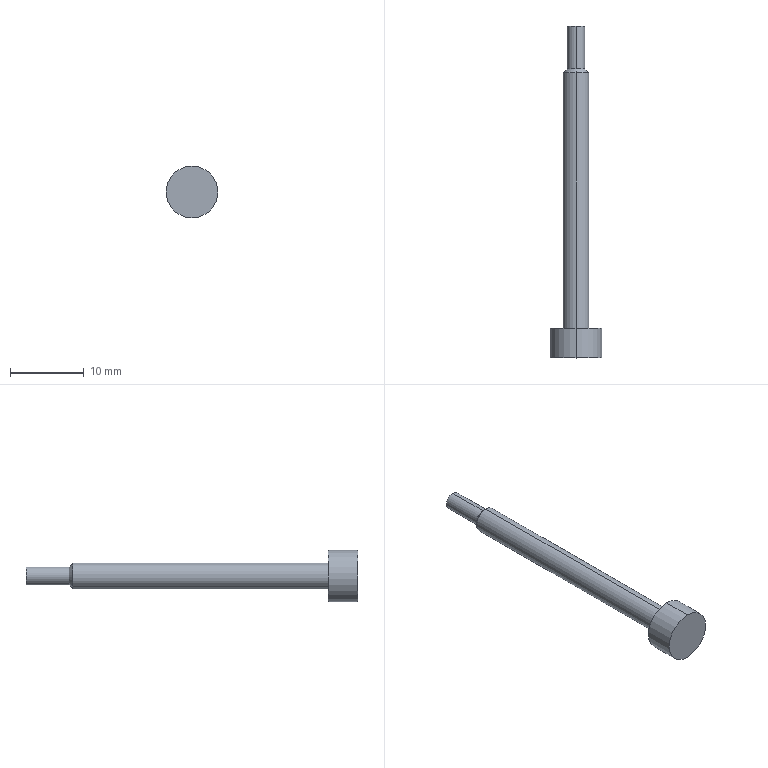Part | STEP file | 1 solid | 12 faces | box 7 x 45.025 x 7 mm | volume 517.748 mm3 | cylinder 6 | plane 4 | cone 2 | commonest cylinder face diameters 2.412 x2 3.5 x2 7 x2
STEP:
#1=CARTESIAN_POINT('',(0.,0.,0.));
#2=DIRECTION('',(0.,0.,1.));
#3=DIRECTION('',(1.,0.,0.));
#4=AXIS2_PLACEMENT_3D('',#1,#2,#3);
#5=CARTESIAN_POINT('',(-135.173,-40.,196.963));
#6=VERTEX_POINT('',#5);
#7=CARTESIAN_POINT('',(-135.173,-40.,189.963));
#8=VERTEX_POINT('',#7);
#9=CARTESIAN_POINT('',(-135.173,-40.,193.463));
#10=DIRECTION('',(0.,1.,0.));
#11=DIRECTION('',(0.,0.,-1.));
#12=AXIS2_PLACEMENT_3D('',#9,#10,#11);
#13=CIRCLE('',#12,3.5);
#14=CARTESIAN_POINT('',(-135.173,-50.,193.463));
#15=DIRECTION('',(0.,1.,0.));
#16=DIRECTION('',(0.,0.,1.));
#17=AXIS2_PLACEMENT_3D('',#14,#15,#16);
#18=CYLINDRICAL_SURFACE('',#17,3.5);
#19=CARTESIAN_POINT('',(-3.142,10.));
#20=DIRECTION('',(1.,0.));
#21=VECTOR('',#20,1.);
#22=LINE('',#19,#21);
#23=(GEOMETRIC_REPRESENTATION_CONTEXT(2)PARAMETRIC_REPRESENTATION_CONTEXT()REPRESENTATION_CONTEXT('',''));
#24=DEFINITIONAL_REPRESENTATION('',(#22),#23);
#25=PCURVE('',#18,#24);
#26=CARTESIAN_POINT('',(-72.862,-40.,23.556));
#27=DIRECTION('',(0.,-1.,0.));
#28=DIRECTION('',(0.,0.,-1.));
#29=AXIS2_PLACEMENT_3D('',#26,#27,#28);
#30=PLANE('',#29);
#31=CARTESIAN_POINT('',(-166.407,-62.31));
#32=CARTESIAN_POINT('',(-166.407,-68.372));
#33=CARTESIAN_POINT('',(-171.657,-65.341));
#34=CARTESIAN_POINT('',(-176.907,-62.31));
#35=CARTESIAN_POINT('',(-171.657,-59.279));
#36=CARTESIAN_POINT('',(-166.407,-56.248));
#37=CARTESIAN_POINT('',(-166.407,-62.31));
#38=(BOUNDED_CURVE()B_SPLINE_CURVE(2,(#31,#32,#33,#34,#35,#36,#37),.UNSPECIFIED.,.T.,.F.)B_SPLINE_CURVE_WITH_KNOTS((1,2,2,2,2,1),(-2.094,0.,2.094,4.189,6.283,8.378),.UNSPECIFIED.)CURVE()GEOMETRIC_REPRESENTATION_ITEM()RATIONAL_B_SPLINE_CURVE((1.,0.5,1.,0.5,1.,0.5,1.))REPRESENTATION_ITEM(''));
#39=(GEOMETRIC_REPRESENTATION_CONTEXT(2)PARAMETRIC_REPRESENTATION_CONTEXT()REPRESENTATION_CONTEXT('',''));
#40=DEFINITIONAL_REPRESENTATION('',(#38),#39);
#41=PCURVE('',#30,#40);
#42=SURFACE_CURVE('',#13,(#25,#41),.PCURVE_S1.);
#43=EDGE_CURVE('',#6,#8,#42,.T.);
#44=ORIENTED_EDGE('',*,*,#43,.T.);
#45=CARTESIAN_POINT('',(-135.173,-36.,189.963));
#46=VERTEX_POINT('',#45);
#47=CARTESIAN_POINT('',(-135.173,-50.,189.963));
#48=DIRECTION('',(0.,1.,0.));
#49=VECTOR('',#48,1.);
#50=LINE('',#47,#49);
#51=CARTESIAN_POINT('',(3.142,0.));
#52=DIRECTION('',(0.,1.));
#53=VECTOR('',#52,1.);
#54=LINE('',#51,#53);
#55=(GEOMETRIC_REPRESENTATION_CONTEXT(2)PARAMETRIC_REPRESENTATION_CONTEXT()REPRESENTATION_CONTEXT('',''));
#56=DEFINITIONAL_REPRESENTATION('',(#54),#55);
#57=PCURVE('',#18,#56);
#58=CARTESIAN_POINT('',(-135.173,-50.,193.463));
#59=DIRECTION('',(0.,1.,0.));
#60=DIRECTION('',(0.,0.,1.));
#61=AXIS2_PLACEMENT_3D('',#58,#59,#60);
#62=CYLINDRICAL_SURFACE('',#61,3.5);
#63=CARTESIAN_POINT('',(3.142,0.));
#64=DIRECTION('',(0.,1.));
#65=VECTOR('',#64,1.);
#66=LINE('',#63,#65);
#67=(GEOMETRIC_REPRESENTATION_CONTEXT(2)PARAMETRIC_REPRESENTATION_CONTEXT()REPRESENTATION_CONTEXT('',''));
#68=DEFINITIONAL_REPRESENTATION('',(#66),#67);
#69=PCURVE('',#62,#68);
#70=SURFACE_CURVE('',#50,(#57,#69),.PCURVE_S1.);
#71=EDGE_CURVE('',#8,#46,#70,.T.);
#72=ORIENTED_EDGE('',*,*,#71,.T.);
#73=CARTESIAN_POINT('',(-135.173,-36.,196.963));
#74=VERTEX_POINT('',#73);
#75=CARTESIAN_POINT('',(-135.173,-36.,193.463));
#76=DIRECTION('',(0.,-1.,0.));
#77=DIRECTION('',(0.,0.,-1.));
#78=AXIS2_PLACEMENT_3D('',#75,#76,#77);
#79=CIRCLE('',#78,3.5);
#80=CARTESIAN_POINT('',(3.142,14.));
#81=DIRECTION('',(-1.,0.));
#82=VECTOR('',#81,1.);
#83=LINE('',#80,#82);
#84=(GEOMETRIC_REPRESENTATION_CONTEXT(2)PARAMETRIC_REPRESENTATION_CONTEXT()REPRESENTATION_CONTEXT('',''));
#85=DEFINITIONAL_REPRESENTATION('',(#83),#84);
#86=PCURVE('',#18,#85);
#87=CARTESIAN_POINT('',(-135.173,-36.,193.463));
#88=DIRECTION('',(0.,1.,0.));
#89=DIRECTION('',(0.,0.,1.));
#90=AXIS2_PLACEMENT_3D('',#87,#88,#89);
#91=PLANE('',#90);
#92=CARTESIAN_POINT('',(-3.5,0.));
#93=CARTESIAN_POINT('',(-3.5,6.062));
#94=CARTESIAN_POINT('',(1.75,3.031));
#95=CARTESIAN_POINT('',(7.,0.));
#96=CARTESIAN_POINT('',(1.75,-3.031));
#97=CARTESIAN_POINT('',(-3.5,-6.062));
#98=CARTESIAN_POINT('',(-3.5,0.));
#99=(BOUNDED_CURVE()B_SPLINE_CURVE(2,(#92,#93,#94,#95,#96,#97,#98),.UNSPECIFIED.,.T.,.F.)B_SPLINE_CURVE_WITH_KNOTS((1,2,2,2,2,1),(-2.094,0.,2.094,4.189,6.283,8.378),.UNSPECIFIED.)CURVE()GEOMETRIC_REPRESENTATION_ITEM()RATIONAL_B_SPLINE_CURVE((1.,0.5,1.,0.5,1.,0.5,1.))REPRESENTATION_ITEM(''));
#100=(GEOMETRIC_REPRESENTATION_CONTEXT(2)PARAMETRIC_REPRESENTATION_CONTEXT()REPRESENTATION_CONTEXT('',''));
#101=DEFINITIONAL_REPRESENTATION('',(#99),#100);
#102=PCURVE('',#91,#101);
#103=SURFACE_CURVE('',#79,(#86,#102),.PCURVE_S1.);
#104=EDGE_CURVE('',#46,#74,#103,.T.);
#105=ORIENTED_EDGE('',*,*,#104,.T.);
#106=CARTESIAN_POINT('',(-135.173,-50.,196.963));
#107=DIRECTION('',(0.,1.,0.));
#108=VECTOR('',#107,1.);
#109=LINE('',#106,#108);
#110=CARTESIAN_POINT('',(0.,0.));
#111=DIRECTION('',(0.,1.));
#112=VECTOR('',#111,1.);
#113=LINE('',#110,#112);
#114=(GEOMETRIC_REPRESENTATION_CONTEXT(2)PARAMETRIC_REPRESENTATION_CONTEXT()REPRESENTATION_CONTEXT('',''));
#115=DEFINITIONAL_REPRESENTATION('',(#113),#114);
#116=PCURVE('',#18,#115);
#117=CARTESIAN_POINT('',(6.283,0.));
#118=DIRECTION('',(0.,1.));
#119=VECTOR('',#118,1.);
#120=LINE('',#117,#119);
#121=(GEOMETRIC_REPRESENTATION_CONTEXT(2)PARAMETRIC_REPRESENTATION_CONTEXT()REPRESENTATION_CONTEXT('',''));
#122=DEFINITIONAL_REPRESENTATION('',(#120),#121);
#123=PCURVE('',#62,#122);
#124=SURFACE_CURVE('',#109,(#116,#123),.PCURVE_S1.);
#125=EDGE_CURVE('',#6,#74,#124,.T.);
#126=ORIENTED_EDGE('',*,*,#125,.F.);
#127=EDGE_LOOP('',(#44,#72,#105,#126));
#128=FACE_BOUND('',#127,.T.);
#129=ADVANCED_FACE('',(#128),#18,.T.);
#130=CARTESIAN_POINT('',(-135.173,-1.306,195.213));
#131=VERTEX_POINT('',#130);
#132=CARTESIAN_POINT('',(-135.173,-1.306,191.713));
#133=VERTEX_POINT('',#132);
#134=CARTESIAN_POINT('',(-135.173,-1.306,193.463));
#135=DIRECTION('',(0.,1.,0.));
#136=DIRECTION('',(0.,0.,-1.));
#137=AXIS2_PLACEMENT_3D('',#134,#135,#136);
#138=CIRCLE('',#137,1.75);
#139=CARTESIAN_POINT('',(-135.173,5.025,193.463));
#140=DIRECTION('',(0.,-1.,0.));
#141=DIRECTION('',(0.,0.,-1.));
#142=AXIS2_PLACEMENT_3D('',#139,#140,#141);
#143=CYLINDRICAL_SURFACE('',#142,1.75);
#144=CARTESIAN_POINT('',(6.283,6.332));
#145=DIRECTION('',(-1.,0.));
#146=VECTOR('',#145,1.);
#147=LINE('',#144,#146);
#148=(GEOMETRIC_REPRESENTATION_CONTEXT(2)PARAMETRIC_REPRESENTATION_CONTEXT()REPRESENTATION_CONTEXT('',''));
#149=DEFINITIONAL_REPRESENTATION('',(#147),#148);
#150=PCURVE('',#143,#149);
#151=CARTESIAN_POINT('',(-134.168,-1.306,193.908));
#152=DIRECTION('',(0.,-1.,0.));
#153=DIRECTION('',(0.,0.,-1.));
#154=AXIS2_PLACEMENT_3D('',#151,#152,#153);
#155=PLANE('',#154);
#156=CARTESIAN_POINT('',(2.196,-1.005));
#157=CARTESIAN_POINT('',(2.196,-4.036));
#158=CARTESIAN_POINT('',(-0.4291,-2.52));
#159=CARTESIAN_POINT('',(-3.054,-1.005));
#160=CARTESIAN_POINT('',(-0.4291,0.5106));
#161=CARTESIAN_POINT('',(2.196,2.026));
#162=CARTESIAN_POINT('',(2.196,-1.005));
#163=(BOUNDED_CURVE()B_SPLINE_CURVE(2,(#156,#157,#158,#159,#160,#161,#162),.UNSPECIFIED.,.T.,.F.)B_SPLINE_CURVE_WITH_KNOTS((1,2,2,2,2,1),(-2.094,0.,2.094,4.189,6.283,8.378),.UNSPECIFIED.)CURVE()GEOMETRIC_REPRESENTATION_ITEM()RATIONAL_B_SPLINE_CURVE((1.,0.5,1.,0.5,1.,0.5,1.))REPRESENTATION_ITEM(''));
#164=(GEOMETRIC_REPRESENTATION_CONTEXT(2)PARAMETRIC_REPRESENTATION_CONTEXT()REPRESENTATION_CONTEXT('',''));
#165=DEFINITIONAL_REPRESENTATION('',(#163),#164);
#166=PCURVE('',#155,#165);
#167=SURFACE_CURVE('',#138,(#150,#166),.PCURVE_S1.);
#168=EDGE_CURVE('',#131,#133,#167,.T.);
#169=ORIENTED_EDGE('',*,*,#168,.F.);
#170=CARTESIAN_POINT('',(-135.173,-36.,195.213));
#171=VERTEX_POINT('',#170);
#172=CARTESIAN_POINT('',(-135.173,5.025,195.213));
#173=DIRECTION('',(0.,-1.,0.));
#174=VECTOR('',#173,1.);
#175=LINE('',#172,#174);
#176=CARTESIAN_POINT('',(3.142,0.));
#177=DIRECTION('',(0.,1.));
#178=VECTOR('',#177,1.);
#179=LINE('',#176,#178);
#180=(GEOMETRIC_REPRESENTATION_CONTEXT(2)PARAMETRIC_REPRESENTATION_CONTEXT()REPRESENTATION_CONTEXT('',''));
#181=DEFINITIONAL_REPRESENTATION('',(#179),#180);
#182=PCURVE('',#143,#181);
#183=CARTESIAN_POINT('',(-135.173,5.025,193.463));
#184=DIRECTION('',(0.,-1.,0.));
#185=DIRECTION('',(0.,0.,-1.));
#186=AXIS2_PLACEMENT_3D('',#183,#184,#185);
#187=CYLINDRICAL_SURFACE('',#186,1.75);
#188=CARTESIAN_POINT('',(3.142,0.));
#189=DIRECTION('',(0.,1.));
#190=VECTOR('',#189,1.);
#191=LINE('',#188,#190);
#192=(GEOMETRIC_REPRESENTATION_CONTEXT(2)PARAMETRIC_REPRESENTATION_CONTEXT()REPRESENTATION_CONTEXT('',''));
#193=DEFINITIONAL_REPRESENTATION('',(#191),#192);
#194=PCURVE('',#187,#193);
#195=SURFACE_CURVE('',#175,(#182,#194),.PCURVE_S1.);
#196=EDGE_CURVE('',#131,#171,#195,.T.);
#197=ORIENTED_EDGE('',*,*,#196,.T.);
#198=CARTESIAN_POINT('',(-135.173,-36.,191.713));
#199=VERTEX_POINT('',#198);
#200=CARTESIAN_POINT('',(-135.173,-36.,193.463));
#201=DIRECTION('',(0.,-1.,0.));
#202=DIRECTION('',(0.,0.,1.));
#203=AXIS2_PLACEMENT_3D('',#200,#201,#202);
#204=CIRCLE('',#203,1.75);
#205=CARTESIAN_POINT('',(-3.142,41.025));
#206=DIRECTION('',(1.,0.));
#207=VECTOR('',#206,1.);
#208=LINE('',#205,#207);
#209=(GEOMETRIC_REPRESENTATION_CONTEXT(2)PARAMETRIC_REPRESENTATION_CONTEXT()REPRESENTATION_CONTEXT('',''));
#210=DEFINITIONAL_REPRESENTATION('',(#208),#209);
#211=PCURVE('',#143,#210);
#212=CARTESIAN_POINT('',(1.75,0.));
#213=CARTESIAN_POINT('',(1.75,-3.031));
#214=CARTESIAN_POINT('',(-0.875,-1.516));
#215=CARTESIAN_POINT('',(-3.5,0.));
#216=CARTESIAN_POINT('',(-0.875,1.516));
#217=CARTESIAN_POINT('',(1.75,3.031));
#218=CARTESIAN_POINT('',(1.75,0.));
#219=(BOUNDED_CURVE()B_SPLINE_CURVE(2,(#212,#213,#214,#215,#216,#217,#218),.UNSPECIFIED.,.T.,.F.)B_SPLINE_CURVE_WITH_KNOTS((1,2,2,2,2,1),(-2.094,0.,2.094,4.189,6.283,8.378),.UNSPECIFIED.)CURVE()GEOMETRIC_REPRESENTATION_ITEM()RATIONAL_B_SPLINE_CURVE((1.,0.5,1.,0.5,1.,0.5,1.))REPRESENTATION_ITEM(''));
#220=(GEOMETRIC_REPRESENTATION_CONTEXT(2)PARAMETRIC_REPRESENTATION_CONTEXT()REPRESENTATION_CONTEXT('',''));
#221=DEFINITIONAL_REPRESENTATION('',(#219),#220);
#222=PCURVE('',#91,#221);
#223=SURFACE_CURVE('',#204,(#211,#222),.PCURVE_S1.);
#224=EDGE_CURVE('',#199,#171,#223,.T.);
#225=ORIENTED_EDGE('',*,*,#224,.F.);
#226=CARTESIAN_POINT('',(-135.173,5.025,191.713));
#227=DIRECTION('',(0.,-1.,0.));
#228=VECTOR('',#227,1.);
#229=LINE('',#226,#228);
#230=CARTESIAN_POINT('',(0.,0.));
#231=DIRECTION('',(0.,1.));
#232=VECTOR('',#231,1.);
#233=LINE('',#230,#232);
#234=(GEOMETRIC_REPRESENTATION_CONTEXT(2)PARAMETRIC_REPRESENTATION_CONTEXT()REPRESENTATION_CONTEXT('',''));
#235=DEFINITIONAL_REPRESENTATION('',(#233),#234);
#236=PCURVE('',#143,#235);
#237=CARTESIAN_POINT('',(6.283,0.));
#238=DIRECTION('',(0.,1.));
#239=VECTOR('',#238,1.);
#240=LINE('',#237,#239);
#241=(GEOMETRIC_REPRESENTATION_CONTEXT(2)PARAMETRIC_REPRESENTATION_CONTEXT()REPRESENTATION_CONTEXT('',''));
#242=DEFINITIONAL_REPRESENTATION('',(#240),#241);
#243=PCURVE('',#187,#242);
#244=SURFACE_CURVE('',#229,(#236,#243),.PCURVE_S1.);
#245=EDGE_CURVE('',#133,#199,#244,.T.);
#246=ORIENTED_EDGE('',*,*,#245,.F.);
#247=EDGE_LOOP('',(#169,#197,#225,#246));
#248=FACE_BOUND('',#247,.T.);
#249=ADVANCED_FACE('',(#248),#143,.T.);
#250=CARTESIAN_POINT('',(-135.173,-0.804,192.256));
#251=VERTEX_POINT('',#250);
#252=CARTESIAN_POINT('',(-135.173,-0.804,194.668));
#253=VERTEX_POINT('',#252);
#254=CARTESIAN_POINT('',(-135.173,-0.804,193.463));
#255=DIRECTION('',(0.,-1.,0.));
#256=DIRECTION('',(0.,0.,-1.));
#257=AXIS2_PLACEMENT_3D('',#254,#255,#256);
#258=CIRCLE('',#257,1.206);
#259=CARTESIAN_POINT('',(-135.173,-1.306,193.463));
#260=DIRECTION('',(0.,-1.,0.));
#261=DIRECTION('',(0.,0.,-1.));
#262=AXIS2_PLACEMENT_3D('',#259,#260,#261);
#263=CONICAL_SURFACE('',#262,1.708,0.7854);
#264=CARTESIAN_POINT('',(0.,-0.5025));
#265=DIRECTION('',(1.,0.));
#266=VECTOR('',#265,1.);
#267=LINE('',#264,#266);
#268=(GEOMETRIC_REPRESENTATION_CONTEXT(2)PARAMETRIC_REPRESENTATION_CONTEXT()REPRESENTATION_CONTEXT('',''));
#269=DEFINITIONAL_REPRESENTATION('',(#267),#268);
#270=PCURVE('',#263,#269);
#271=CARTESIAN_POINT('',(-135.173,90.286,193.463));
#272=DIRECTION('',(0.,-1.,0.));
#273=DIRECTION('',(0.,0.,-1.));
#274=AXIS2_PLACEMENT_3D('',#271,#272,#273);
#275=CYLINDRICAL_SURFACE('',#274,1.206);
#276=CARTESIAN_POINT('',(0.,91.09));
#277=DIRECTION('',(1.,0.));
#278=VECTOR('',#277,1.);
#279=LINE('',#276,#278);
#280=(GEOMETRIC_REPRESENTATION_CONTEXT(2)PARAMETRIC_REPRESENTATION_CONTEXT()REPRESENTATION_CONTEXT('',''));
#281=DEFINITIONAL_REPRESENTATION('',(#279),#280);
#282=PCURVE('',#275,#281);
#283=SURFACE_CURVE('',#258,(#270,#282),.PCURVE_S1.);
#284=EDGE_CURVE('',#251,#253,#283,.T.);
#285=ORIENTED_EDGE('',*,*,#284,.T.);
#286=CARTESIAN_POINT('',(-135.173,-1.306,195.171));
#287=VERTEX_POINT('',#286);
#288=CARTESIAN_POINT('',(-135.173,-1.306,195.171));
#289=DIRECTION('',(0.,-0.7071,0.7071));
#290=VECTOR('',#289,1.);
#291=LINE('',#288,#290);
#292=CARTESIAN_POINT('',(3.142,0.));
#293=DIRECTION('',(0.,1.));
#294=VECTOR('',#293,1.);
#295=LINE('',#292,#294);
#296=(GEOMETRIC_REPRESENTATION_CONTEXT(2)PARAMETRIC_REPRESENTATION_CONTEXT()REPRESENTATION_CONTEXT('',''));
#297=DEFINITIONAL_REPRESENTATION('',(#295),#296);
#298=PCURVE('',#263,#297);
#299=CARTESIAN_POINT('',(-135.173,-1.306,193.463));
#300=DIRECTION('',(0.,-1.,0.));
#301=DIRECTION('',(0.,0.,-1.));
#302=AXIS2_PLACEMENT_3D('',#299,#300,#301);
#303=CONICAL_SURFACE('',#302,1.708,0.7854);
#304=CARTESIAN_POINT('',(3.142,0.));
#305=DIRECTION('',(0.,1.));
#306=VECTOR('',#305,1.);
#307=LINE('',#304,#306);
#308=(GEOMETRIC_REPRESENTATION_CONTEXT(2)PARAMETRIC_REPRESENTATION_CONTEXT()REPRESENTATION_CONTEXT('',''));
#309=DEFINITIONAL_REPRESENTATION('',(#307),#308);
#310=PCURVE('',#303,#309);
#311=SURFACE_CURVE('',#291,(#298,#310),.PCURVE_S1.);
#312=EDGE_CURVE('',#253,#287,#311,.T.);
#313=ORIENTED_EDGE('',*,*,#312,.T.);
#314=CARTESIAN_POINT('',(-135.173,-1.306,191.754));
#315=VERTEX_POINT('',#314);
#316=CARTESIAN_POINT('',(-135.173,-1.306,193.463));
#317=DIRECTION('',(0.,1.,0.));
#318=DIRECTION('',(0.,0.,-1.));
#319=AXIS2_PLACEMENT_3D('',#316,#317,#318);
#320=CIRCLE('',#319,1.708);
#321=CARTESIAN_POINT('',(6.283,0.));
#322=DIRECTION('',(-1.,0.));
#323=VECTOR('',#322,1.);
#324=LINE('',#321,#323);
#325=(GEOMETRIC_REPRESENTATION_CONTEXT(2)PARAMETRIC_REPRESENTATION_CONTEXT()REPRESENTATION_CONTEXT('',''));
#326=DEFINITIONAL_REPRESENTATION('',(#324),#325);
#327=PCURVE('',#263,#326);
#328=CARTESIAN_POINT('',(2.154,-1.005));
#329=CARTESIAN_POINT('',(2.154,-3.964));
#330=CARTESIAN_POINT('',(-0.4083,-2.485));
#331=CARTESIAN_POINT('',(-2.971,-1.005));
#332=CARTESIAN_POINT('',(-0.4083,0.4747));
#333=CARTESIAN_POINT('',(2.154,1.954));
#334=CARTESIAN_POINT('',(2.154,-1.005));
#335=(BOUNDED_CURVE()B_SPLINE_CURVE(2,(#328,#329,#330,#331,#332,#333,#334),.UNSPECIFIED.,.T.,.F.)B_SPLINE_CURVE_WITH_KNOTS((1,2,2,2,2,1),(-2.094,0.,2.094,4.189,6.283,8.378),.UNSPECIFIED.)CURVE()GEOMETRIC_REPRESENTATION_ITEM()RATIONAL_B_SPLINE_CURVE((1.,0.5,1.,0.5,1.,0.5,1.))REPRESENTATION_ITEM(''));
#336=(GEOMETRIC_REPRESENTATION_CONTEXT(2)PARAMETRIC_REPRESENTATION_CONTEXT()REPRESENTATION_CONTEXT('',''));
#337=DEFINITIONAL_REPRESENTATION('',(#335),#336);
#338=PCURVE('',#155,#337);
#339=SURFACE_CURVE('',#320,(#327,#338),.PCURVE_S1.);
#340=EDGE_CURVE('',#287,#315,#339,.T.);
#341=ORIENTED_EDGE('',*,*,#340,.T.);
#342=CARTESIAN_POINT('',(-135.173,-1.306,191.754));
#343=DIRECTION('',(0.,-0.7071,-0.7071));
#344=VECTOR('',#343,1.);
#345=LINE('',#342,#344);
#346=CARTESIAN_POINT('',(0.,0.));
#347=DIRECTION('',(0.,1.));
#348=VECTOR('',#347,1.);
#349=LINE('',#346,#348);
#350=(GEOMETRIC_REPRESENTATION_CONTEXT(2)PARAMETRIC_REPRESENTATION_CONTEXT()REPRESENTATION_CONTEXT('',''));
#351=DEFINITIONAL_REPRESENTATION('',(#349),#350);
#352=PCURVE('',#263,#351);
#353=CARTESIAN_POINT('',(6.283,0.));
#354=DIRECTION('',(0.,1.));
#355=VECTOR('',#354,1.);
#356=LINE('',#353,#355);
#357=(GEOMETRIC_REPRESENTATION_CONTEXT(2)PARAMETRIC_REPRESENTATION_CONTEXT()REPRESENTATION_CONTEXT('',''));
#358=DEFINITIONAL_REPRESENTATION('',(#356),#357);
#359=PCURVE('',#303,#358);
#360=SURFACE_CURVE('',#345,(#352,#359),.PCURVE_S1.);
#361=EDGE_CURVE('',#251,#315,#360,.T.);
#362=ORIENTED_EDGE('',*,*,#361,.F.);
#363=EDGE_LOOP('',(#285,#313,#341,#362));
#364=FACE_BOUND('',#363,.T.);
#365=ADVANCED_FACE('',(#364),#263,.T.);
#366=CARTESIAN_POINT('',(-135.173,5.025,194.668));
#367=VERTEX_POINT('',#366);
#368=CARTESIAN_POINT('',(-135.173,5.025,192.256));
#369=VERTEX_POINT('',#368);
#370=CARTESIAN_POINT('',(-135.173,5.025,193.463));
#371=DIRECTION('',(0.,1.,0.));
#372=DIRECTION('',(0.,0.,1.));
#373=AXIS2_PLACEMENT_3D('',#370,#371,#372);
#374=CIRCLE('',#373,1.206);
#375=CARTESIAN_POINT('',(3.142,85.261));
#376=DIRECTION('',(-1.,0.));
#377=VECTOR('',#376,1.);
#378=LINE('',#375,#377);
#379=(GEOMETRIC_REPRESENTATION_CONTEXT(2)PARAMETRIC_REPRESENTATION_CONTEXT()REPRESENTATION_CONTEXT('',''));
#380=DEFINITIONAL_REPRESENTATION('',(#378),#379);
#381=PCURVE('',#275,#380);
#382=CARTESIAN_POINT('',(-135.173,5.025,193.463));
#383=DIRECTION('',(0.,1.,0.));
#384=DIRECTION('',(0.,0.,1.));
#385=AXIS2_PLACEMENT_3D('',#382,#383,#384);
#386=PLANE('',#385);
#387=CARTESIAN_POINT('',(0.,0.));
#388=DIRECTION('',(1.,0.));
#389=AXIS2_PLACEMENT_2D('',#387,#388);
#390=CIRCLE('',#389,1.206);
#391=(GEOMETRIC_REPRESENTATION_CONTEXT(2)PARAMETRIC_REPRESENTATION_CONTEXT()REPRESENTATION_CONTEXT('',''));
#392=DEFINITIONAL_REPRESENTATION('',(#390),#391);
#393=PCURVE('',#386,#392);
#394=SURFACE_CURVE('',#374,(#381,#393),.PCURVE_S1.);
#395=EDGE_CURVE('',#367,#369,#394,.T.);
#396=ORIENTED_EDGE('',*,*,#395,.F.);
#397=CARTESIAN_POINT('',(-135.173,90.286,194.668));
#398=DIRECTION('',(0.,-1.,0.));
#399=VECTOR('',#398,1.);
#400=LINE('',#397,#399);
#401=CARTESIAN_POINT('',(3.142,0.));
#402=DIRECTION('',(0.,1.));
#403=VECTOR('',#402,1.);
#404=LINE('',#401,#403);
#405=(GEOMETRIC_REPRESENTATION_CONTEXT(2)PARAMETRIC_REPRESENTATION_CONTEXT()REPRESENTATION_CONTEXT('',''));
#406=DEFINITIONAL_REPRESENTATION('',(#404),#405);
#407=PCURVE('',#275,#406);
#408=CARTESIAN_POINT('',(-135.173,90.286,193.463));
#409=DIRECTION('',(0.,-1.,0.));
#410=DIRECTION('',(0.,0.,-1.));
#411=AXIS2_PLACEMENT_3D('',#408,#409,#410);
#412=CYLINDRICAL_SURFACE('',#411,1.206);
#413=CARTESIAN_POINT('',(3.142,0.));
#414=DIRECTION('',(0.,1.));
#415=VECTOR('',#414,1.);
#416=LINE('',#413,#415);
#417=(GEOMETRIC_REPRESENTATION_CONTEXT(2)PARAMETRIC_REPRESENTATION_CONTEXT()REPRESENTATION_CONTEXT('',''));
#418=DEFINITIONAL_REPRESENTATION('',(#416),#417);
#419=PCURVE('',#412,#418);
#420=SURFACE_CURVE('',#400,(#407,#419),.PCURVE_S1.);
#421=EDGE_CURVE('',#367,#253,#420,.T.);
#422=ORIENTED_EDGE('',*,*,#421,.T.);
#423=ORIENTED_EDGE('',*,*,#284,.F.);
#424=CARTESIAN_POINT('',(-135.173,90.286,192.256));
#425=DIRECTION('',(0.,-1.,0.));
#426=VECTOR('',#425,1.);
#427=LINE('',#424,#426);
#428=CARTESIAN_POINT('',(0.,0.));
#429=DIRECTION('',(0.,1.));
#430=VECTOR('',#429,1.);
#431=LINE('',#428,#430);
#432=(GEOMETRIC_REPRESENTATION_CONTEXT(2)PARAMETRIC_REPRESENTATION_CONTEXT()REPRESENTATION_CONTEXT('',''));
#433=DEFINITIONAL_REPRESENTATION('',(#431),#432);
#434=PCURVE('',#275,#433);
#435=CARTESIAN_POINT('',(6.283,0.));
#436=DIRECTION('',(0.,1.));
#437=VECTOR('',#436,1.);
#438=LINE('',#435,#437);
#439=(GEOMETRIC_REPRESENTATION_CONTEXT(2)PARAMETRIC_REPRESENTATION_CONTEXT()REPRESENTATION_CONTEXT('',''));
#440=DEFINITIONAL_REPRESENTATION('',(#438),#439);
#441=PCURVE('',#412,#440);
#442=SURFACE_CURVE('',#427,(#434,#441),.PCURVE_S1.);
#443=EDGE_CURVE('',#369,#251,#442,.T.);
#444=ORIENTED_EDGE('',*,*,#443,.F.);
#445=EDGE_LOOP('',(#396,#422,#423,#444));
#446=FACE_BOUND('',#445,.T.);
#447=ADVANCED_FACE('',(#446),#275,.T.);
#448=ORIENTED_EDGE('',*,*,#421,.F.);
#449=CARTESIAN_POINT('',(-135.173,5.025,193.463));
#450=DIRECTION('',(0.,1.,0.));
#451=DIRECTION('',(0.,0.,1.));
#452=AXIS2_PLACEMENT_3D('',#449,#450,#451);
#453=CIRCLE('',#452,1.206);
#454=CARTESIAN_POINT('',(9.425,85.261));
#455=DIRECTION('',(-1.,0.));
#456=VECTOR('',#455,1.);
#457=LINE('',#454,#456);
#458=(GEOMETRIC_REPRESENTATION_CONTEXT(2)PARAMETRIC_REPRESENTATION_CONTEXT()REPRESENTATION_CONTEXT('',''));
#459=DEFINITIONAL_REPRESENTATION('',(#457),#458);
#460=PCURVE('',#412,#459);
#461=CARTESIAN_POINT('',(0.,0.));
#462=DIRECTION('',(1.,0.));
#463=AXIS2_PLACEMENT_2D('',#461,#462);
#464=CIRCLE('',#463,1.206);
#465=(GEOMETRIC_REPRESENTATION_CONTEXT(2)PARAMETRIC_REPRESENTATION_CONTEXT()REPRESENTATION_CONTEXT('',''));
#466=DEFINITIONAL_REPRESENTATION('',(#464),#465);
#467=PCURVE('',#386,#466);
#468=SURFACE_CURVE('',#453,(#460,#467),.PCURVE_S1.);
#469=EDGE_CURVE('',#369,#367,#468,.T.);
#470=ORIENTED_EDGE('',*,*,#469,.F.);
#471=ORIENTED_EDGE('',*,*,#443,.T.);
#472=CARTESIAN_POINT('',(-135.173,-0.804,193.463));
#473=DIRECTION('',(0.,-1.,0.));
#474=DIRECTION('',(0.,0.,-1.));
#475=AXIS2_PLACEMENT_3D('',#472,#473,#474);
#476=CIRCLE('',#475,1.206);
#477=CARTESIAN_POINT('',(0.,91.09));
#478=DIRECTION('',(1.,0.));
#479=VECTOR('',#478,1.);
#480=LINE('',#477,#479);
#481=(GEOMETRIC_REPRESENTATION_CONTEXT(2)PARAMETRIC_REPRESENTATION_CONTEXT()REPRESENTATION_CONTEXT('',''));
#482=DEFINITIONAL_REPRESENTATION('',(#480),#481);
#483=PCURVE('',#412,#482);
#484=CARTESIAN_POINT('',(0.,-0.5025));
#485=DIRECTION('',(1.,0.));
#486=VECTOR('',#485,1.);
#487=LINE('',#484,#486);
#488=(GEOMETRIC_REPRESENTATION_CONTEXT(2)PARAMETRIC_REPRESENTATION_CONTEXT()REPRESENTATION_CONTEXT('',''));
#489=DEFINITIONAL_REPRESENTATION('',(#487),#488);
#490=PCURVE('',#303,#489);
#491=SURFACE_CURVE('',#476,(#483,#490),.PCURVE_S1.);
#492=EDGE_CURVE('',#253,#251,#491,.T.);
#493=ORIENTED_EDGE('',*,*,#492,.F.);
#494=EDGE_LOOP('',(#448,#470,#471,#493));
#495=FACE_BOUND('',#494,.T.);
#496=ADVANCED_FACE('',(#495),#412,.T.);
#497=ORIENTED_EDGE('',*,*,#312,.F.);
#498=ORIENTED_EDGE('',*,*,#492,.T.);
#499=ORIENTED_EDGE('',*,*,#361,.T.);
#500=CARTESIAN_POINT('',(-135.173,-1.306,193.463));
#501=DIRECTION('',(0.,1.,0.));
#502=DIRECTION('',(0.,0.,-1.));
#503=AXIS2_PLACEMENT_3D('',#500,#501,#502);
#504=CIRCLE('',#503,1.708);
#505=CARTESIAN_POINT('',(6.283,0.));
#506=DIRECTION('',(-1.,0.));
#507=VECTOR('',#506,1.);
#508=LINE('',#505,#507);
#509=(GEOMETRIC_REPRESENTATION_CONTEXT(2)PARAMETRIC_REPRESENTATION_CONTEXT()REPRESENTATION_CONTEXT('',''));
#510=DEFINITIONAL_REPRESENTATION('',(#508),#509);
#511=PCURVE('',#303,#510);
#512=CARTESIAN_POINT('',(2.154,-1.005));
#513=CARTESIAN_POINT('',(2.154,-3.964));
#514=CARTESIAN_POINT('',(-0.4083,-2.485));
#515=CARTESIAN_POINT('',(-2.971,-1.005));
#516=CARTESIAN_POINT('',(-0.4083,0.4747));
#517=CARTESIAN_POINT('',(2.154,1.954));
#518=CARTESIAN_POINT('',(2.154,-1.005));
#519=(BOUNDED_CURVE()B_SPLINE_CURVE(2,(#512,#513,#514,#515,#516,#517,#518),.UNSPECIFIED.,.T.,.F.)B_SPLINE_CURVE_WITH_KNOTS((1,2,2,2,2,1),(-2.094,0.,2.094,4.189,6.283,8.378),.UNSPECIFIED.)CURVE()GEOMETRIC_REPRESENTATION_ITEM()RATIONAL_B_SPLINE_CURVE((1.,0.5,1.,0.5,1.,0.5,1.))REPRESENTATION_ITEM(''));
#520=(GEOMETRIC_REPRESENTATION_CONTEXT(2)PARAMETRIC_REPRESENTATION_CONTEXT()REPRESENTATION_CONTEXT('',''));
#521=DEFINITIONAL_REPRESENTATION('',(#519),#520);
#522=PCURVE('',#155,#521);
#523=SURFACE_CURVE('',#504,(#511,#522),.PCURVE_S1.);
#524=EDGE_CURVE('',#315,#287,#523,.T.);
#525=ORIENTED_EDGE('',*,*,#524,.T.);
#526=EDGE_LOOP('',(#497,#498,#499,#525));
#527=FACE_BOUND('',#526,.T.);
#528=ADVANCED_FACE('',(#527),#303,.T.);
#529=CARTESIAN_POINT('',(-135.173,-1.306,193.463));
#530=DIRECTION('',(0.,1.,0.));
#531=DIRECTION('',(0.,0.,-1.));
#532=AXIS2_PLACEMENT_3D('',#529,#530,#531);
#533=CIRCLE('',#532,1.75);
#534=CARTESIAN_POINT('',(2.196,-1.005));
#535=CARTESIAN_POINT('',(2.196,-4.036));
#536=CARTESIAN_POINT('',(-0.4291,-2.52));
#537=CARTESIAN_POINT('',(-3.054,-1.005));
#538=CARTESIAN_POINT('',(-0.4291,0.5106));
#539=CARTESIAN_POINT('',(2.196,2.026));
#540=CARTESIAN_POINT('',(2.196,-1.005));
#541=(BOUNDED_CURVE()B_SPLINE_CURVE(2,(#534,#535,#536,#537,#538,#539,#540),.UNSPECIFIED.,.T.,.F.)B_SPLINE_CURVE_WITH_KNOTS((1,2,2,2,2,1),(-2.094,0.,2.094,4.189,6.283,8.378),.UNSPECIFIED.)CURVE()GEOMETRIC_REPRESENTATION_ITEM()RATIONAL_B_SPLINE_CURVE((1.,0.5,1.,0.5,1.,0.5,1.))REPRESENTATION_ITEM(''));
#542=(GEOMETRIC_REPRESENTATION_CONTEXT(2)PARAMETRIC_REPRESENTATION_CONTEXT()REPRESENTATION_CONTEXT('',''));
#543=DEFINITIONAL_REPRESENTATION('',(#541),#542);
#544=PCURVE('',#155,#543);
#545=CARTESIAN_POINT('',(6.283,6.332));
#546=DIRECTION('',(-1.,0.));
#547=VECTOR('',#546,1.);
#548=LINE('',#545,#547);
#549=(GEOMETRIC_REPRESENTATION_CONTEXT(2)PARAMETRIC_REPRESENTATION_CONTEXT()REPRESENTATION_CONTEXT('',''));
#550=DEFINITIONAL_REPRESENTATION('',(#548),#549);
#551=PCURVE('',#187,#550);
#552=SURFACE_CURVE('',#533,(#544,#551),.PCURVE_S1.);
#553=EDGE_CURVE('',#133,#131,#552,.T.);
#554=ORIENTED_EDGE('',*,*,#553,.T.);
#555=ORIENTED_EDGE('',*,*,#168,.T.);
#556=EDGE_LOOP('',(#554,#555));
#557=FACE_BOUND('',#556,.T.);
#558=ORIENTED_EDGE('',*,*,#524,.F.);
#559=ORIENTED_EDGE('',*,*,#340,.F.);
#560=EDGE_LOOP('',(#558,#559));
#561=FACE_BOUND('',#560,.T.);
#562=ADVANCED_FACE('',(#557,#561),#155,.F.);
#563=ORIENTED_EDGE('',*,*,#196,.F.);
#564=ORIENTED_EDGE('',*,*,#553,.F.);
#565=ORIENTED_EDGE('',*,*,#245,.T.);
#566=CARTESIAN_POINT('',(-135.173,-36.,193.463));
#567=DIRECTION('',(0.,-1.,0.));
#568=DIRECTION('',(0.,0.,1.));
#569=AXIS2_PLACEMENT_3D('',#566,#567,#568);
#570=CIRCLE('',#569,1.75);
#571=CARTESIAN_POINT('',(3.142,41.025));
#572=DIRECTION('',(1.,0.));
#573=VECTOR('',#572,1.);
#574=LINE('',#571,#573);
#575=(GEOMETRIC_REPRESENTATION_CONTEXT(2)PARAMETRIC_REPRESENTATION_CONTEXT()REPRESENTATION_CONTEXT('',''));
#576=DEFINITIONAL_REPRESENTATION('',(#574),#575);
#577=PCURVE('',#187,#576);
#578=CARTESIAN_POINT('',(1.75,0.));
#579=CARTESIAN_POINT('',(1.75,-3.031));
#580=CARTESIAN_POINT('',(-0.875,-1.516));
#581=CARTESIAN_POINT('',(-3.5,0.));
#582=CARTESIAN_POINT('',(-0.875,1.516));
#583=CARTESIAN_POINT('',(1.75,3.031));
#584=CARTESIAN_POINT('',(1.75,0.));
#585=(BOUNDED_CURVE()B_SPLINE_CURVE(2,(#578,#579,#580,#581,#582,#583,#584),.UNSPECIFIED.,.T.,.F.)B_SPLINE_CURVE_WITH_KNOTS((1,2,2,2,2,1),(-2.094,0.,2.094,4.189,6.283,8.378),.UNSPECIFIED.)CURVE()GEOMETRIC_REPRESENTATION_ITEM()RATIONAL_B_SPLINE_CURVE((1.,0.5,1.,0.5,1.,0.5,1.))REPRESENTATION_ITEM(''));
#586=(GEOMETRIC_REPRESENTATION_CONTEXT(2)PARAMETRIC_REPRESENTATION_CONTEXT()REPRESENTATION_CONTEXT('',''));
#587=DEFINITIONAL_REPRESENTATION('',(#585),#586);
#588=PCURVE('',#91,#587);
#589=SURFACE_CURVE('',#570,(#577,#588),.PCURVE_S1.);
#590=EDGE_CURVE('',#171,#199,#589,.T.);
#591=ORIENTED_EDGE('',*,*,#590,.F.);
#592=EDGE_LOOP('',(#563,#564,#565,#591));
#593=FACE_BOUND('',#592,.T.);
#594=ADVANCED_FACE('',(#593),#187,.T.);
#595=ORIENTED_EDGE('',*,*,#469,.T.);
#596=ORIENTED_EDGE('',*,*,#395,.T.);
#597=EDGE_LOOP('',(#595,#596));
#598=FACE_BOUND('',#597,.T.);
#599=ADVANCED_FACE('',(#598),#386,.T.);
#600=ORIENTED_EDGE('',*,*,#224,.T.);
#601=ORIENTED_EDGE('',*,*,#590,.T.);
#602=EDGE_LOOP('',(#600,#601));
#603=FACE_BOUND('',#602,.T.);
#604=CARTESIAN_POINT('',(-135.173,-36.,193.463));
#605=DIRECTION('',(0.,-1.,0.));
#606=DIRECTION('',(0.,0.,-1.));
#607=AXIS2_PLACEMENT_3D('',#604,#605,#606);
#608=CIRCLE('',#607,3.5);
#609=CARTESIAN_POINT('',(-3.5,0.));
#610=CARTESIAN_POINT('',(-3.5,6.062));
#611=CARTESIAN_POINT('',(1.75,3.031));
#612=CARTESIAN_POINT('',(7.,0.));
#613=CARTESIAN_POINT('',(1.75,-3.031));
#614=CARTESIAN_POINT('',(-3.5,-6.062));
#615=CARTESIAN_POINT('',(-3.5,0.));
#616=(BOUNDED_CURVE()B_SPLINE_CURVE(2,(#609,#610,#611,#612,#613,#614,#615),.UNSPECIFIED.,.T.,.F.)B_SPLINE_CURVE_WITH_KNOTS((1,2,2,2,2,1),(-2.094,0.,2.094,4.189,6.283,8.378),.UNSPECIFIED.)CURVE()GEOMETRIC_REPRESENTATION_ITEM()RATIONAL_B_SPLINE_CURVE((1.,0.5,1.,0.5,1.,0.5,1.))REPRESENTATION_ITEM(''));
#617=(GEOMETRIC_REPRESENTATION_CONTEXT(2)PARAMETRIC_REPRESENTATION_CONTEXT()REPRESENTATION_CONTEXT('',''));
#618=DEFINITIONAL_REPRESENTATION('',(#616),#617);
#619=PCURVE('',#91,#618);
#620=CARTESIAN_POINT('',(9.425,14.));
#621=DIRECTION('',(-1.,0.));
#622=VECTOR('',#621,1.);
#623=LINE('',#620,#622);
#624=(GEOMETRIC_REPRESENTATION_CONTEXT(2)PARAMETRIC_REPRESENTATION_CONTEXT()REPRESENTATION_CONTEXT('',''));
#625=DEFINITIONAL_REPRESENTATION('',(#623),#624);
#626=PCURVE('',#62,#625);
#627=SURFACE_CURVE('',#608,(#619,#626),.PCURVE_S1.);
#628=EDGE_CURVE('',#74,#46,#627,.T.);
#629=ORIENTED_EDGE('',*,*,#628,.F.);
#630=ORIENTED_EDGE('',*,*,#104,.F.);
#631=EDGE_LOOP('',(#629,#630));
#632=FACE_BOUND('',#631,.T.);
#633=ADVANCED_FACE('',(#603,#632),#91,.T.);
#634=ORIENTED_EDGE('',*,*,#71,.F.);
#635=CARTESIAN_POINT('',(-135.173,-40.,193.463));
#636=DIRECTION('',(0.,1.,0.));
#637=DIRECTION('',(0.,0.,-1.));
#638=AXIS2_PLACEMENT_3D('',#635,#636,#637);
#639=CIRCLE('',#638,3.5);
#640=CARTESIAN_POINT('',(3.142,10.));
#641=DIRECTION('',(1.,0.));
#642=VECTOR('',#641,1.);
#643=LINE('',#640,#642);
#644=(GEOMETRIC_REPRESENTATION_CONTEXT(2)PARAMETRIC_REPRESENTATION_CONTEXT()REPRESENTATION_CONTEXT('',''));
#645=DEFINITIONAL_REPRESENTATION('',(#643),#644);
#646=PCURVE('',#62,#645);
#647=CARTESIAN_POINT('',(-166.407,-62.31));
#648=CARTESIAN_POINT('',(-166.407,-68.372));
#649=CARTESIAN_POINT('',(-171.657,-65.341));
#650=CARTESIAN_POINT('',(-176.907,-62.31));
#651=CARTESIAN_POINT('',(-171.657,-59.279));
#652=CARTESIAN_POINT('',(-166.407,-56.248));
#653=CARTESIAN_POINT('',(-166.407,-62.31));
#654=(BOUNDED_CURVE()B_SPLINE_CURVE(2,(#647,#648,#649,#650,#651,#652,#653),.UNSPECIFIED.,.T.,.F.)B_SPLINE_CURVE_WITH_KNOTS((1,2,2,2,2,1),(-2.094,0.,2.094,4.189,6.283,8.378),.UNSPECIFIED.)CURVE()GEOMETRIC_REPRESENTATION_ITEM()RATIONAL_B_SPLINE_CURVE((1.,0.5,1.,0.5,1.,0.5,1.))REPRESENTATION_ITEM(''));
#655=(GEOMETRIC_REPRESENTATION_CONTEXT(2)PARAMETRIC_REPRESENTATION_CONTEXT()REPRESENTATION_CONTEXT('',''));
#656=DEFINITIONAL_REPRESENTATION('',(#654),#655);
#657=PCURVE('',#30,#656);
#658=SURFACE_CURVE('',#639,(#646,#657),.PCURVE_S1.);
#659=EDGE_CURVE('',#8,#6,#658,.T.);
#660=ORIENTED_EDGE('',*,*,#659,.T.);
#661=ORIENTED_EDGE('',*,*,#125,.T.);
#662=ORIENTED_EDGE('',*,*,#628,.T.);
#663=EDGE_LOOP('',(#634,#660,#661,#662));
#664=FACE_BOUND('',#663,.T.);
#665=ADVANCED_FACE('',(#664),#62,.T.);
#666=ORIENTED_EDGE('',*,*,#43,.F.);
#667=ORIENTED_EDGE('',*,*,#659,.F.);
#668=EDGE_LOOP('',(#666,#667));
#669=FACE_BOUND('',#668,.T.);
#670=ADVANCED_FACE('',(#669),#30,.T.);
#671=CLOSED_SHELL('',(#129,#249,#365,#447,#496,#528,#562,#594,#599,#633,#665,#670));
#672=MANIFOLD_SOLID_BREP('',#671);
#673=(LENGTH_UNIT()NAMED_UNIT(*)SI_UNIT(.MILLI.,.METRE.));
#674=UNCERTAINTY_MEASURE_WITH_UNIT(LENGTH_MEASURE(0.0000001),#673,'','');
#675=(NAMED_UNIT(*)PLANE_ANGLE_UNIT()SI_UNIT($,.RADIAN.));
#676=(NAMED_UNIT(*)SI_UNIT($,.STERADIAN.)SOLID_ANGLE_UNIT());
#677=(GEOMETRIC_REPRESENTATION_CONTEXT(3)GLOBAL_UNCERTAINTY_ASSIGNED_CONTEXT((#674))GLOBAL_UNIT_ASSIGNED_CONTEXT((#673,#675,#676))REPRESENTATION_CONTEXT('',''));
#678=ADVANCED_BREP_SHAPE_REPRESENTATION('',(#4,#672),#677);